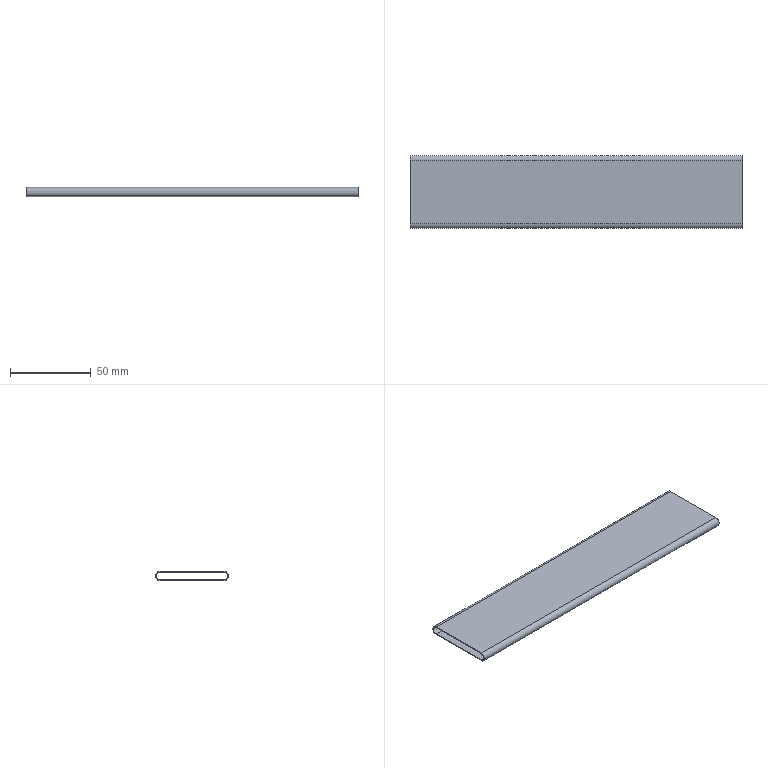Part | STEP file | Tube feed_id914_x_t | 1 solid | 10 faces | box 205 x 45.1 x 5.7 mm | volume 9751 mm3 | plane 6 | cylinder 4 | commonest cylinder face diameters 4.7 x2 5.7 x2
STEP:
#1=CARTESIAN_POINT('',(0.,0.,0.));
#2=DIRECTION('',(0.,0.,1.));
#3=DIRECTION('',(1.,0.,0.));
#4=AXIS2_PLACEMENT_3D('',#1,#2,#3);
#5=CARTESIAN_POINT('',(-74.,-9.664,-6.));
#6=VERTEX_POINT('',#5);
#7=CARTESIAN_POINT('',(-74.,29.736,-6.));
#8=VERTEX_POINT('',#7);
#9=CARTESIAN_POINT('',(-74.,-9.664,-6.));
#10=DIRECTION('',(0.,1.,0.));
#11=VECTOR('',#10,1.);
#12=LINE('',#9,#11);
#13=CARTESIAN_POINT('',(231.,-9.664,-6.));
#14=DIRECTION('',(0.,0.,1.));
#15=DIRECTION('',(0.,-1.,0.));
#16=AXIS2_PLACEMENT_3D('',#13,#14,#15);
#17=PLANE('',#16);
#18=CARTESIAN_POINT('',(0.,-305.));
#19=DIRECTION('',(-1.,0.));
#20=VECTOR('',#19,1.);
#21=LINE('',#18,#20);
#22=(GEOMETRIC_REPRESENTATION_CONTEXT(2)PARAMETRIC_REPRESENTATION_CONTEXT()REPRESENTATION_CONTEXT('',''));
#23=DEFINITIONAL_REPRESENTATION('',(#21),#22);
#24=PCURVE('',#17,#23);
#25=CARTESIAN_POINT('',(-74.,29.736,-3.15));
#26=DIRECTION('',(1.,0.,0.));
#27=DIRECTION('',(0.,0.,-1.));
#28=AXIS2_PLACEMENT_3D('',#25,#26,#27);
#29=PLANE('',#28);
#30=CARTESIAN_POINT('',(2.85,-39.4));
#31=DIRECTION('',(0.,1.));
#32=VECTOR('',#31,1.);
#33=LINE('',#30,#32);
#34=(GEOMETRIC_REPRESENTATION_CONTEXT(2)PARAMETRIC_REPRESENTATION_CONTEXT()REPRESENTATION_CONTEXT('',''));
#35=DEFINITIONAL_REPRESENTATION('',(#33),#34);
#36=PCURVE('',#29,#35);
#37=SURFACE_CURVE('',#12,(#24,#36),.PCURVE_S1.);
#38=EDGE_CURVE('',#6,#8,#37,.T.);
#39=ORIENTED_EDGE('',*,*,#38,.T.);
#40=CARTESIAN_POINT('',(131.,29.736,-6.));
#41=VERTEX_POINT('',#40);
#42=CARTESIAN_POINT('',(231.,29.736,-6.));
#43=DIRECTION('',(-1.,0.,0.));
#44=VECTOR('',#43,1.);
#45=LINE('',#42,#44);
#46=CARTESIAN_POINT('',(-39.4,0.));
#47=DIRECTION('',(0.,-1.));
#48=VECTOR('',#47,1.);
#49=LINE('',#46,#48);
#50=(GEOMETRIC_REPRESENTATION_CONTEXT(2)PARAMETRIC_REPRESENTATION_CONTEXT()REPRESENTATION_CONTEXT('',''));
#51=DEFINITIONAL_REPRESENTATION('',(#49),#50);
#52=PCURVE('',#17,#51);
#53=CARTESIAN_POINT('',(231.,29.736,-3.15));
#54=DIRECTION('',(-1.,0.,0.));
#55=DIRECTION('',(0.,-1.,0.));
#56=AXIS2_PLACEMENT_3D('',#53,#54,#55);
#57=CYLINDRICAL_SURFACE('',#56,2.85);
#58=CARTESIAN_POINT('',(4.712,0.));
#59=DIRECTION('',(0.,1.));
#60=VECTOR('',#59,1.);
#61=LINE('',#58,#60);
#62=(GEOMETRIC_REPRESENTATION_CONTEXT(2)PARAMETRIC_REPRESENTATION_CONTEXT()REPRESENTATION_CONTEXT('',''));
#63=DEFINITIONAL_REPRESENTATION('',(#61),#62);
#64=PCURVE('',#57,#63);
#65=SURFACE_CURVE('',#45,(#52,#64),.PCURVE_S1.);
#66=EDGE_CURVE('',#41,#8,#65,.T.);
#67=ORIENTED_EDGE('',*,*,#66,.F.);
#68=CARTESIAN_POINT('',(131.,-9.664,-6.));
#69=VERTEX_POINT('',#68);
#70=CARTESIAN_POINT('',(131.,-9.664,-6.));
#71=DIRECTION('',(0.,1.,0.));
#72=VECTOR('',#71,1.);
#73=LINE('',#70,#72);
#74=CARTESIAN_POINT('',(0.,-100.));
#75=DIRECTION('',(-1.,0.));
#76=VECTOR('',#75,1.);
#77=LINE('',#74,#76);
#78=(GEOMETRIC_REPRESENTATION_CONTEXT(2)PARAMETRIC_REPRESENTATION_CONTEXT()REPRESENTATION_CONTEXT('',''));
#79=DEFINITIONAL_REPRESENTATION('',(#77),#78);
#80=PCURVE('',#17,#79);
#81=CARTESIAN_POINT('',(131.,29.736,-3.15));
#82=DIRECTION('',(1.,0.,0.));
#83=DIRECTION('',(0.,0.,-1.));
#84=AXIS2_PLACEMENT_3D('',#81,#82,#83);
#85=PLANE('',#84);
#86=CARTESIAN_POINT('',(2.85,-39.4));
#87=DIRECTION('',(0.,1.));
#88=VECTOR('',#87,1.);
#89=LINE('',#86,#88);
#90=(GEOMETRIC_REPRESENTATION_CONTEXT(2)PARAMETRIC_REPRESENTATION_CONTEXT()REPRESENTATION_CONTEXT('',''));
#91=DEFINITIONAL_REPRESENTATION('',(#89),#90);
#92=PCURVE('',#85,#91);
#93=SURFACE_CURVE('',#73,(#80,#92),.PCURVE_S1.);
#94=EDGE_CURVE('',#69,#41,#93,.T.);
#95=ORIENTED_EDGE('',*,*,#94,.F.);
#96=CARTESIAN_POINT('',(231.,-9.664,-6.));
#97=DIRECTION('',(-1.,0.,0.));
#98=VECTOR('',#97,1.);
#99=LINE('',#96,#98);
#100=CARTESIAN_POINT('',(0.,0.));
#101=DIRECTION('',(0.,-1.));
#102=VECTOR('',#101,1.);
#103=LINE('',#100,#102);
#104=(GEOMETRIC_REPRESENTATION_CONTEXT(2)PARAMETRIC_REPRESENTATION_CONTEXT()REPRESENTATION_CONTEXT('',''));
#105=DEFINITIONAL_REPRESENTATION('',(#103),#104);
#106=PCURVE('',#17,#105);
#107=CARTESIAN_POINT('',(231.,-9.664,-3.15));
#108=DIRECTION('',(-1.,0.,0.));
#109=DIRECTION('',(0.,-1.,0.));
#110=AXIS2_PLACEMENT_3D('',#107,#108,#109);
#111=CYLINDRICAL_SURFACE('',#110,2.85);
#112=CARTESIAN_POINT('',(-1.571,0.));
#113=DIRECTION('',(0.,1.));
#114=VECTOR('',#113,1.);
#115=LINE('',#112,#114);
#116=(GEOMETRIC_REPRESENTATION_CONTEXT(2)PARAMETRIC_REPRESENTATION_CONTEXT()REPRESENTATION_CONTEXT('',''));
#117=DEFINITIONAL_REPRESENTATION('',(#115),#116);
#118=PCURVE('',#111,#117);
#119=SURFACE_CURVE('',#99,(#106,#118),.PCURVE_S1.);
#120=EDGE_CURVE('',#69,#6,#119,.T.);
#121=ORIENTED_EDGE('',*,*,#120,.T.);
#122=EDGE_LOOP('',(#39,#67,#95,#121));
#123=FACE_BOUND('',#122,.T.);
#124=ADVANCED_FACE('',(#123),#17,.F.);
#125=CARTESIAN_POINT('',(-74.,29.736,-0.3));
#126=VERTEX_POINT('',#125);
#127=CARTESIAN_POINT('',(-74.,29.736,-3.15));
#128=DIRECTION('',(1.,0.,0.));
#129=DIRECTION('',(0.,1.,0.));
#130=AXIS2_PLACEMENT_3D('',#127,#128,#129);
#131=CIRCLE('',#130,2.85);
#132=CARTESIAN_POINT('',(9.425,305.));
#133=DIRECTION('',(-1.,0.));
#134=VECTOR('',#133,1.);
#135=LINE('',#132,#134);
#136=(GEOMETRIC_REPRESENTATION_CONTEXT(2)PARAMETRIC_REPRESENTATION_CONTEXT()REPRESENTATION_CONTEXT('',''));
#137=DEFINITIONAL_REPRESENTATION('',(#135),#136);
#138=PCURVE('',#57,#137);
#139=CARTESIAN_POINT('',(0.,0.));
#140=DIRECTION('',(0.,1.));
#141=AXIS2_PLACEMENT_2D('',#139,#140);
#142=CIRCLE('',#141,2.85);
#143=(GEOMETRIC_REPRESENTATION_CONTEXT(2)PARAMETRIC_REPRESENTATION_CONTEXT()REPRESENTATION_CONTEXT('',''));
#144=DEFINITIONAL_REPRESENTATION('',(#142),#143);
#145=PCURVE('',#29,#144);
#146=SURFACE_CURVE('',#131,(#138,#145),.PCURVE_S1.);
#147=EDGE_CURVE('',#8,#126,#146,.T.);
#148=ORIENTED_EDGE('',*,*,#147,.T.);
#149=CARTESIAN_POINT('',(131.,29.736,-0.3));
#150=VERTEX_POINT('',#149);
#151=CARTESIAN_POINT('',(231.,29.736,-0.3));
#152=DIRECTION('',(-1.,0.,0.));
#153=VECTOR('',#152,1.);
#154=LINE('',#151,#153);
#155=CARTESIAN_POINT('',(1.571,0.));
#156=DIRECTION('',(0.,1.));
#157=VECTOR('',#156,1.);
#158=LINE('',#155,#157);
#159=(GEOMETRIC_REPRESENTATION_CONTEXT(2)PARAMETRIC_REPRESENTATION_CONTEXT()REPRESENTATION_CONTEXT('',''));
#160=DEFINITIONAL_REPRESENTATION('',(#158),#159);
#161=PCURVE('',#57,#160);
#162=CARTESIAN_POINT('',(231.,29.736,-0.3));
#163=DIRECTION('',(0.,0.,-1.));
#164=DIRECTION('',(0.,1.,0.));
#165=AXIS2_PLACEMENT_3D('',#162,#163,#164);
#166=PLANE('',#165);
#167=CARTESIAN_POINT('',(0.,0.));
#168=DIRECTION('',(0.,-1.));
#169=VECTOR('',#168,1.);
#170=LINE('',#167,#169);
#171=(GEOMETRIC_REPRESENTATION_CONTEXT(2)PARAMETRIC_REPRESENTATION_CONTEXT()REPRESENTATION_CONTEXT('',''));
#172=DEFINITIONAL_REPRESENTATION('',(#170),#171);
#173=PCURVE('',#166,#172);
#174=SURFACE_CURVE('',#154,(#161,#173),.PCURVE_S1.);
#175=EDGE_CURVE('',#150,#126,#174,.T.);
#176=ORIENTED_EDGE('',*,*,#175,.F.);
#177=CARTESIAN_POINT('',(131.,29.736,-3.15));
#178=DIRECTION('',(1.,0.,0.));
#179=DIRECTION('',(0.,0.,-1.));
#180=AXIS2_PLACEMENT_3D('',#177,#178,#179);
#181=CIRCLE('',#180,2.85);
#182=CARTESIAN_POINT('',(4.712,100.));
#183=DIRECTION('',(-1.,0.));
#184=VECTOR('',#183,1.);
#185=LINE('',#182,#184);
#186=(GEOMETRIC_REPRESENTATION_CONTEXT(2)PARAMETRIC_REPRESENTATION_CONTEXT()REPRESENTATION_CONTEXT('',''));
#187=DEFINITIONAL_REPRESENTATION('',(#185),#186);
#188=PCURVE('',#57,#187);
#189=CARTESIAN_POINT('',(0.,0.));
#190=DIRECTION('',(1.,0.));
#191=AXIS2_PLACEMENT_2D('',#189,#190);
#192=CIRCLE('',#191,2.85);
#193=(GEOMETRIC_REPRESENTATION_CONTEXT(2)PARAMETRIC_REPRESENTATION_CONTEXT()REPRESENTATION_CONTEXT('',''));
#194=DEFINITIONAL_REPRESENTATION('',(#192),#193);
#195=PCURVE('',#85,#194);
#196=SURFACE_CURVE('',#181,(#188,#195),.PCURVE_S1.);
#197=EDGE_CURVE('',#41,#150,#196,.T.);
#198=ORIENTED_EDGE('',*,*,#197,.F.);
#199=ORIENTED_EDGE('',*,*,#66,.T.);
#200=EDGE_LOOP('',(#148,#176,#198,#199));
#201=FACE_BOUND('',#200,.T.);
#202=ADVANCED_FACE('',(#201),#57,.T.);
#203=CARTESIAN_POINT('',(-74.,-9.664,-0.3));
#204=VERTEX_POINT('',#203);
#205=CARTESIAN_POINT('',(-74.,29.736,-0.3));
#206=DIRECTION('',(0.,-1.,0.));
#207=VECTOR('',#206,1.);
#208=LINE('',#205,#207);
#209=CARTESIAN_POINT('',(0.,-305.));
#210=DIRECTION('',(-1.,0.));
#211=VECTOR('',#210,1.);
#212=LINE('',#209,#211);
#213=(GEOMETRIC_REPRESENTATION_CONTEXT(2)PARAMETRIC_REPRESENTATION_CONTEXT()REPRESENTATION_CONTEXT('',''));
#214=DEFINITIONAL_REPRESENTATION('',(#212),#213);
#215=PCURVE('',#166,#214);
#216=CARTESIAN_POINT('',(-2.85,0.));
#217=DIRECTION('',(0.,-1.));
#218=VECTOR('',#217,1.);
#219=LINE('',#216,#218);
#220=(GEOMETRIC_REPRESENTATION_CONTEXT(2)PARAMETRIC_REPRESENTATION_CONTEXT()REPRESENTATION_CONTEXT('',''));
#221=DEFINITIONAL_REPRESENTATION('',(#219),#220);
#222=PCURVE('',#29,#221);
#223=SURFACE_CURVE('',#208,(#215,#222),.PCURVE_S1.);
#224=EDGE_CURVE('',#126,#204,#223,.T.);
#225=ORIENTED_EDGE('',*,*,#224,.T.);
#226=CARTESIAN_POINT('',(131.,-9.664,-0.3));
#227=VERTEX_POINT('',#226);
#228=CARTESIAN_POINT('',(231.,-9.664,-0.3));
#229=DIRECTION('',(-1.,0.,0.));
#230=VECTOR('',#229,1.);
#231=LINE('',#228,#230);
#232=CARTESIAN_POINT('',(-39.4,0.));
#233=DIRECTION('',(0.,-1.));
#234=VECTOR('',#233,1.);
#235=LINE('',#232,#234);
#236=(GEOMETRIC_REPRESENTATION_CONTEXT(2)PARAMETRIC_REPRESENTATION_CONTEXT()REPRESENTATION_CONTEXT('',''));
#237=DEFINITIONAL_REPRESENTATION('',(#235),#236);
#238=PCURVE('',#166,#237);
#239=CARTESIAN_POINT('',(1.571,0.));
#240=DIRECTION('',(0.,1.));
#241=VECTOR('',#240,1.);
#242=LINE('',#239,#241);
#243=(GEOMETRIC_REPRESENTATION_CONTEXT(2)PARAMETRIC_REPRESENTATION_CONTEXT()REPRESENTATION_CONTEXT('',''));
#244=DEFINITIONAL_REPRESENTATION('',(#242),#243);
#245=PCURVE('',#111,#244);
#246=SURFACE_CURVE('',#231,(#238,#245),.PCURVE_S1.);
#247=EDGE_CURVE('',#227,#204,#246,.T.);
#248=ORIENTED_EDGE('',*,*,#247,.F.);
#249=CARTESIAN_POINT('',(131.,29.736,-0.3));
#250=DIRECTION('',(0.,-1.,0.));
#251=VECTOR('',#250,1.);
#252=LINE('',#249,#251);
#253=CARTESIAN_POINT('',(0.,-100.));
#254=DIRECTION('',(-1.,0.));
#255=VECTOR('',#254,1.);
#256=LINE('',#253,#255);
#257=(GEOMETRIC_REPRESENTATION_CONTEXT(2)PARAMETRIC_REPRESENTATION_CONTEXT()REPRESENTATION_CONTEXT('',''));
#258=DEFINITIONAL_REPRESENTATION('',(#256),#257);
#259=PCURVE('',#166,#258);
#260=CARTESIAN_POINT('',(-2.85,0.));
#261=DIRECTION('',(0.,-1.));
#262=VECTOR('',#261,1.);
#263=LINE('',#260,#262);
#264=(GEOMETRIC_REPRESENTATION_CONTEXT(2)PARAMETRIC_REPRESENTATION_CONTEXT()REPRESENTATION_CONTEXT('',''));
#265=DEFINITIONAL_REPRESENTATION('',(#263),#264);
#266=PCURVE('',#85,#265);
#267=SURFACE_CURVE('',#252,(#259,#266),.PCURVE_S1.);
#268=EDGE_CURVE('',#150,#227,#267,.T.);
#269=ORIENTED_EDGE('',*,*,#268,.F.);
#270=ORIENTED_EDGE('',*,*,#175,.T.);
#271=EDGE_LOOP('',(#225,#248,#269,#270));
#272=FACE_BOUND('',#271,.T.);
#273=ADVANCED_FACE('',(#272),#166,.F.);
#274=CARTESIAN_POINT('',(-74.,-9.664,-3.15));
#275=DIRECTION('',(1.,0.,0.));
#276=DIRECTION('',(0.,1.,0.));
#277=AXIS2_PLACEMENT_3D('',#274,#275,#276);
#278=CIRCLE('',#277,2.85);
#279=CARTESIAN_POINT('',(3.142,305.));
#280=DIRECTION('',(-1.,0.));
#281=VECTOR('',#280,1.);
#282=LINE('',#279,#281);
#283=(GEOMETRIC_REPRESENTATION_CONTEXT(2)PARAMETRIC_REPRESENTATION_CONTEXT()REPRESENTATION_CONTEXT('',''));
#284=DEFINITIONAL_REPRESENTATION('',(#282),#283);
#285=PCURVE('',#111,#284);
#286=CARTESIAN_POINT('',(0.,-39.4));
#287=DIRECTION('',(0.,1.));
#288=AXIS2_PLACEMENT_2D('',#286,#287);
#289=CIRCLE('',#288,2.85);
#290=(GEOMETRIC_REPRESENTATION_CONTEXT(2)PARAMETRIC_REPRESENTATION_CONTEXT()REPRESENTATION_CONTEXT('',''));
#291=DEFINITIONAL_REPRESENTATION('',(#289),#290);
#292=PCURVE('',#29,#291);
#293=SURFACE_CURVE('',#278,(#285,#292),.PCURVE_S1.);
#294=EDGE_CURVE('',#204,#6,#293,.T.);
#295=ORIENTED_EDGE('',*,*,#294,.T.);
#296=ORIENTED_EDGE('',*,*,#120,.F.);
#297=CARTESIAN_POINT('',(131.,-9.664,-3.15));
#298=DIRECTION('',(1.,0.,0.));
#299=DIRECTION('',(0.,0.,-1.));
#300=AXIS2_PLACEMENT_3D('',#297,#298,#299);
#301=CIRCLE('',#300,2.85);
#302=CARTESIAN_POINT('',(4.712,100.));
#303=DIRECTION('',(-1.,0.));
#304=VECTOR('',#303,1.);
#305=LINE('',#302,#304);
#306=(GEOMETRIC_REPRESENTATION_CONTEXT(2)PARAMETRIC_REPRESENTATION_CONTEXT()REPRESENTATION_CONTEXT('',''));
#307=DEFINITIONAL_REPRESENTATION('',(#305),#306);
#308=PCURVE('',#111,#307);
#309=CARTESIAN_POINT('',(0.,-39.4));
#310=DIRECTION('',(1.,0.));
#311=AXIS2_PLACEMENT_2D('',#309,#310);
#312=CIRCLE('',#311,2.85);
#313=(GEOMETRIC_REPRESENTATION_CONTEXT(2)PARAMETRIC_REPRESENTATION_CONTEXT()REPRESENTATION_CONTEXT('',''));
#314=DEFINITIONAL_REPRESENTATION('',(#312),#313);
#315=PCURVE('',#85,#314);
#316=SURFACE_CURVE('',#301,(#308,#315),.PCURVE_S1.);
#317=EDGE_CURVE('',#227,#69,#316,.T.);
#318=ORIENTED_EDGE('',*,*,#317,.F.);
#319=ORIENTED_EDGE('',*,*,#247,.T.);
#320=EDGE_LOOP('',(#295,#296,#318,#319));
#321=FACE_BOUND('',#320,.T.);
#322=ADVANCED_FACE('',(#321),#111,.T.);
#323=CARTESIAN_POINT('',(131.,-9.664,-5.5));
#324=VERTEX_POINT('',#323);
#325=CARTESIAN_POINT('',(131.,29.736,-5.5));
#326=VERTEX_POINT('',#325);
#327=CARTESIAN_POINT('',(131.,-9.664,-5.5));
#328=DIRECTION('',(0.,1.,0.));
#329=VECTOR('',#328,1.);
#330=LINE('',#327,#329);
#331=CARTESIAN_POINT('',(2.35,-39.4));
#332=DIRECTION('',(0.,1.));
#333=VECTOR('',#332,1.);
#334=LINE('',#331,#333);
#335=(GEOMETRIC_REPRESENTATION_CONTEXT(2)PARAMETRIC_REPRESENTATION_CONTEXT()REPRESENTATION_CONTEXT('',''));
#336=DEFINITIONAL_REPRESENTATION('',(#334),#335);
#337=PCURVE('',#85,#336);
#338=CARTESIAN_POINT('',(231.,-9.664,-5.5));
#339=DIRECTION('',(0.,0.,1.));
#340=DIRECTION('',(0.,-1.,0.));
#341=AXIS2_PLACEMENT_3D('',#338,#339,#340);
#342=PLANE('',#341);
#343=CARTESIAN_POINT('',(0.,-100.));
#344=DIRECTION('',(-1.,0.));
#345=VECTOR('',#344,1.);
#346=LINE('',#343,#345);
#347=(GEOMETRIC_REPRESENTATION_CONTEXT(2)PARAMETRIC_REPRESENTATION_CONTEXT()REPRESENTATION_CONTEXT('',''));
#348=DEFINITIONAL_REPRESENTATION('',(#346),#347);
#349=PCURVE('',#342,#348);
#350=SURFACE_CURVE('',#330,(#337,#349),.PCURVE_S1.);
#351=EDGE_CURVE('',#324,#326,#350,.T.);
#352=ORIENTED_EDGE('',*,*,#351,.F.);
#353=CARTESIAN_POINT('',(131.,-9.664,-0.8));
#354=VERTEX_POINT('',#353);
#355=CARTESIAN_POINT('',(131.,-9.664,-3.15));
#356=DIRECTION('',(1.,0.,0.));
#357=DIRECTION('',(0.,0.,-1.));
#358=AXIS2_PLACEMENT_3D('',#355,#356,#357);
#359=CIRCLE('',#358,2.35);
#360=CARTESIAN_POINT('',(0.,-39.4));
#361=DIRECTION('',(1.,0.));
#362=AXIS2_PLACEMENT_2D('',#360,#361);
#363=CIRCLE('',#362,2.35);
#364=(GEOMETRIC_REPRESENTATION_CONTEXT(2)PARAMETRIC_REPRESENTATION_CONTEXT()REPRESENTATION_CONTEXT('',''));
#365=DEFINITIONAL_REPRESENTATION('',(#363),#364);
#366=PCURVE('',#85,#365);
#367=CARTESIAN_POINT('',(231.,-9.664,-3.15));
#368=DIRECTION('',(-1.,0.,0.));
#369=DIRECTION('',(0.,-1.,0.));
#370=AXIS2_PLACEMENT_3D('',#367,#368,#369);
#371=CYLINDRICAL_SURFACE('',#370,2.35);
#372=CARTESIAN_POINT('',(10.996,100.));
#373=DIRECTION('',(-1.,0.));
#374=VECTOR('',#373,1.);
#375=LINE('',#372,#374);
#376=(GEOMETRIC_REPRESENTATION_CONTEXT(2)PARAMETRIC_REPRESENTATION_CONTEXT()REPRESENTATION_CONTEXT('',''));
#377=DEFINITIONAL_REPRESENTATION('',(#375),#376);
#378=PCURVE('',#371,#377);
#379=SURFACE_CURVE('',#359,(#366,#378),.PCURVE_S1.);
#380=EDGE_CURVE('',#354,#324,#379,.T.);
#381=ORIENTED_EDGE('',*,*,#380,.F.);
#382=CARTESIAN_POINT('',(131.,29.736,-0.8));
#383=VERTEX_POINT('',#382);
#384=CARTESIAN_POINT('',(131.,29.736,-0.8));
#385=DIRECTION('',(0.,-1.,0.));
#386=VECTOR('',#385,1.);
#387=LINE('',#384,#386);
#388=CARTESIAN_POINT('',(-2.35,0.));
#389=DIRECTION('',(0.,-1.));
#390=VECTOR('',#389,1.);
#391=LINE('',#388,#390);
#392=(GEOMETRIC_REPRESENTATION_CONTEXT(2)PARAMETRIC_REPRESENTATION_CONTEXT()REPRESENTATION_CONTEXT('',''));
#393=DEFINITIONAL_REPRESENTATION('',(#391),#392);
#394=PCURVE('',#85,#393);
#395=CARTESIAN_POINT('',(231.,29.736,-0.8));
#396=DIRECTION('',(0.,0.,-1.));
#397=DIRECTION('',(0.,1.,0.));
#398=AXIS2_PLACEMENT_3D('',#395,#396,#397);
#399=PLANE('',#398);
#400=CARTESIAN_POINT('',(0.,-100.));
#401=DIRECTION('',(-1.,0.));
#402=VECTOR('',#401,1.);
#403=LINE('',#400,#402);
#404=(GEOMETRIC_REPRESENTATION_CONTEXT(2)PARAMETRIC_REPRESENTATION_CONTEXT()REPRESENTATION_CONTEXT('',''));
#405=DEFINITIONAL_REPRESENTATION('',(#403),#404);
#406=PCURVE('',#399,#405);
#407=SURFACE_CURVE('',#387,(#394,#406),.PCURVE_S1.);
#408=EDGE_CURVE('',#383,#354,#407,.T.);
#409=ORIENTED_EDGE('',*,*,#408,.F.);
#410=CARTESIAN_POINT('',(131.,29.736,-3.15));
#411=DIRECTION('',(1.,0.,0.));
#412=DIRECTION('',(0.,0.,-1.));
#413=AXIS2_PLACEMENT_3D('',#410,#411,#412);
#414=CIRCLE('',#413,2.35);
#415=CARTESIAN_POINT('',(0.,0.));
#416=DIRECTION('',(1.,0.));
#417=AXIS2_PLACEMENT_2D('',#415,#416);
#418=CIRCLE('',#417,2.35);
#419=(GEOMETRIC_REPRESENTATION_CONTEXT(2)PARAMETRIC_REPRESENTATION_CONTEXT()REPRESENTATION_CONTEXT('',''));
#420=DEFINITIONAL_REPRESENTATION('',(#418),#419);
#421=PCURVE('',#85,#420);
#422=CARTESIAN_POINT('',(231.,29.736,-3.15));
#423=DIRECTION('',(-1.,0.,0.));
#424=DIRECTION('',(0.,-1.,0.));
#425=AXIS2_PLACEMENT_3D('',#422,#423,#424);
#426=CYLINDRICAL_SURFACE('',#425,2.35);
#427=CARTESIAN_POINT('',(4.712,100.));
#428=DIRECTION('',(-1.,0.));
#429=VECTOR('',#428,1.);
#430=LINE('',#427,#429);
#431=(GEOMETRIC_REPRESENTATION_CONTEXT(2)PARAMETRIC_REPRESENTATION_CONTEXT()REPRESENTATION_CONTEXT('',''));
#432=DEFINITIONAL_REPRESENTATION('',(#430),#431);
#433=PCURVE('',#426,#432);
#434=SURFACE_CURVE('',#414,(#421,#433),.PCURVE_S1.);
#435=EDGE_CURVE('',#326,#383,#434,.T.);
#436=ORIENTED_EDGE('',*,*,#435,.F.);
#437=EDGE_LOOP('',(#352,#381,#409,#436));
#438=FACE_BOUND('',#437,.T.);
#439=ORIENTED_EDGE('',*,*,#94,.T.);
#440=ORIENTED_EDGE('',*,*,#197,.T.);
#441=ORIENTED_EDGE('',*,*,#268,.T.);
#442=ORIENTED_EDGE('',*,*,#317,.T.);
#443=EDGE_LOOP('',(#439,#440,#441,#442));
#444=FACE_BOUND('',#443,.T.);
#445=ADVANCED_FACE('',(#438,#444),#85,.T.);
#446=CARTESIAN_POINT('',(-74.,-9.664,-0.8));
#447=VERTEX_POINT('',#446);
#448=CARTESIAN_POINT('',(-74.,-9.664,-5.5));
#449=VERTEX_POINT('',#448);
#450=CARTESIAN_POINT('',(-74.,-9.664,-3.15));
#451=DIRECTION('',(1.,0.,0.));
#452=DIRECTION('',(0.,0.,-1.));
#453=AXIS2_PLACEMENT_3D('',#450,#451,#452);
#454=CIRCLE('',#453,2.35);
#455=CARTESIAN_POINT('',(0.,-39.4));
#456=DIRECTION('',(1.,0.));
#457=AXIS2_PLACEMENT_2D('',#455,#456);
#458=CIRCLE('',#457,2.35);
#459=(GEOMETRIC_REPRESENTATION_CONTEXT(2)PARAMETRIC_REPRESENTATION_CONTEXT()REPRESENTATION_CONTEXT('',''));
#460=DEFINITIONAL_REPRESENTATION('',(#458),#459);
#461=PCURVE('',#29,#460);
#462=CARTESIAN_POINT('',(10.996,305.));
#463=DIRECTION('',(-1.,0.));
#464=VECTOR('',#463,1.);
#465=LINE('',#462,#464);
#466=(GEOMETRIC_REPRESENTATION_CONTEXT(2)PARAMETRIC_REPRESENTATION_CONTEXT()REPRESENTATION_CONTEXT('',''));
#467=DEFINITIONAL_REPRESENTATION('',(#465),#466);
#468=PCURVE('',#371,#467);
#469=SURFACE_CURVE('',#454,(#461,#468),.PCURVE_S1.);
#470=EDGE_CURVE('',#447,#449,#469,.T.);
#471=ORIENTED_EDGE('',*,*,#470,.T.);
#472=CARTESIAN_POINT('',(-74.,29.736,-5.5));
#473=VERTEX_POINT('',#472);
#474=CARTESIAN_POINT('',(-74.,-9.664,-5.5));
#475=DIRECTION('',(0.,1.,0.));
#476=VECTOR('',#475,1.);
#477=LINE('',#474,#476);
#478=CARTESIAN_POINT('',(2.35,-39.4));
#479=DIRECTION('',(0.,1.));
#480=VECTOR('',#479,1.);
#481=LINE('',#478,#480);
#482=(GEOMETRIC_REPRESENTATION_CONTEXT(2)PARAMETRIC_REPRESENTATION_CONTEXT()REPRESENTATION_CONTEXT('',''));
#483=DEFINITIONAL_REPRESENTATION('',(#481),#482);
#484=PCURVE('',#29,#483);
#485=CARTESIAN_POINT('',(0.,-305.));
#486=DIRECTION('',(-1.,0.));
#487=VECTOR('',#486,1.);
#488=LINE('',#485,#487);
#489=(GEOMETRIC_REPRESENTATION_CONTEXT(2)PARAMETRIC_REPRESENTATION_CONTEXT()REPRESENTATION_CONTEXT('',''));
#490=DEFINITIONAL_REPRESENTATION('',(#488),#489);
#491=PCURVE('',#342,#490);
#492=SURFACE_CURVE('',#477,(#484,#491),.PCURVE_S1.);
#493=EDGE_CURVE('',#449,#473,#492,.T.);
#494=ORIENTED_EDGE('',*,*,#493,.T.);
#495=CARTESIAN_POINT('',(-74.,29.736,-0.8));
#496=VERTEX_POINT('',#495);
#497=CARTESIAN_POINT('',(-74.,29.736,-3.15));
#498=DIRECTION('',(1.,0.,0.));
#499=DIRECTION('',(0.,0.,-1.));
#500=AXIS2_PLACEMENT_3D('',#497,#498,#499);
#501=CIRCLE('',#500,2.35);
#502=CARTESIAN_POINT('',(0.,0.));
#503=DIRECTION('',(1.,0.));
#504=AXIS2_PLACEMENT_2D('',#502,#503);
#505=CIRCLE('',#504,2.35);
#506=(GEOMETRIC_REPRESENTATION_CONTEXT(2)PARAMETRIC_REPRESENTATION_CONTEXT()REPRESENTATION_CONTEXT('',''));
#507=DEFINITIONAL_REPRESENTATION('',(#505),#506);
#508=PCURVE('',#29,#507);
#509=CARTESIAN_POINT('',(4.712,305.));
#510=DIRECTION('',(-1.,0.));
#511=VECTOR('',#510,1.);
#512=LINE('',#509,#511);
#513=(GEOMETRIC_REPRESENTATION_CONTEXT(2)PARAMETRIC_REPRESENTATION_CONTEXT()REPRESENTATION_CONTEXT('',''));
#514=DEFINITIONAL_REPRESENTATION('',(#512),#513);
#515=PCURVE('',#426,#514);
#516=SURFACE_CURVE('',#501,(#508,#515),.PCURVE_S1.);
#517=EDGE_CURVE('',#473,#496,#516,.T.);
#518=ORIENTED_EDGE('',*,*,#517,.T.);
#519=CARTESIAN_POINT('',(-74.,29.736,-0.8));
#520=DIRECTION('',(0.,-1.,0.));
#521=VECTOR('',#520,1.);
#522=LINE('',#519,#521);
#523=CARTESIAN_POINT('',(-2.35,0.));
#524=DIRECTION('',(0.,-1.));
#525=VECTOR('',#524,1.);
#526=LINE('',#523,#525);
#527=(GEOMETRIC_REPRESENTATION_CONTEXT(2)PARAMETRIC_REPRESENTATION_CONTEXT()REPRESENTATION_CONTEXT('',''));
#528=DEFINITIONAL_REPRESENTATION('',(#526),#527);
#529=PCURVE('',#29,#528);
#530=CARTESIAN_POINT('',(0.,-305.));
#531=DIRECTION('',(-1.,0.));
#532=VECTOR('',#531,1.);
#533=LINE('',#530,#532);
#534=(GEOMETRIC_REPRESENTATION_CONTEXT(2)PARAMETRIC_REPRESENTATION_CONTEXT()REPRESENTATION_CONTEXT('',''));
#535=DEFINITIONAL_REPRESENTATION('',(#533),#534);
#536=PCURVE('',#399,#535);
#537=SURFACE_CURVE('',#522,(#529,#536),.PCURVE_S1.);
#538=EDGE_CURVE('',#496,#447,#537,.T.);
#539=ORIENTED_EDGE('',*,*,#538,.T.);
#540=EDGE_LOOP('',(#471,#494,#518,#539));
#541=FACE_BOUND('',#540,.T.);
#542=ORIENTED_EDGE('',*,*,#38,.F.);
#543=ORIENTED_EDGE('',*,*,#294,.F.);
#544=ORIENTED_EDGE('',*,*,#224,.F.);
#545=ORIENTED_EDGE('',*,*,#147,.F.);
#546=EDGE_LOOP('',(#542,#543,#544,#545));
#547=FACE_BOUND('',#546,.T.);
#548=ADVANCED_FACE('',(#541,#547),#29,.F.);
#549=ORIENTED_EDGE('',*,*,#493,.F.);
#550=CARTESIAN_POINT('',(231.,-9.664,-5.5));
#551=DIRECTION('',(-1.,0.,0.));
#552=VECTOR('',#551,1.);
#553=LINE('',#550,#552);
#554=CARTESIAN_POINT('',(0.,0.));
#555=DIRECTION('',(0.,-1.));
#556=VECTOR('',#555,1.);
#557=LINE('',#554,#556);
#558=(GEOMETRIC_REPRESENTATION_CONTEXT(2)PARAMETRIC_REPRESENTATION_CONTEXT()REPRESENTATION_CONTEXT('',''));
#559=DEFINITIONAL_REPRESENTATION('',(#557),#558);
#560=PCURVE('',#342,#559);
#561=CARTESIAN_POINT('',(4.712,0.));
#562=DIRECTION('',(0.,1.));
#563=VECTOR('',#562,1.);
#564=LINE('',#561,#563);
#565=(GEOMETRIC_REPRESENTATION_CONTEXT(2)PARAMETRIC_REPRESENTATION_CONTEXT()REPRESENTATION_CONTEXT('',''));
#566=DEFINITIONAL_REPRESENTATION('',(#564),#565);
#567=PCURVE('',#371,#566);
#568=SURFACE_CURVE('',#553,(#560,#567),.PCURVE_S1.);
#569=EDGE_CURVE('',#324,#449,#568,.T.);
#570=ORIENTED_EDGE('',*,*,#569,.F.);
#571=ORIENTED_EDGE('',*,*,#351,.T.);
#572=CARTESIAN_POINT('',(231.,29.736,-5.5));
#573=DIRECTION('',(-1.,0.,0.));
#574=VECTOR('',#573,1.);
#575=LINE('',#572,#574);
#576=CARTESIAN_POINT('',(-39.4,0.));
#577=DIRECTION('',(0.,-1.));
#578=VECTOR('',#577,1.);
#579=LINE('',#576,#578);
#580=(GEOMETRIC_REPRESENTATION_CONTEXT(2)PARAMETRIC_REPRESENTATION_CONTEXT()REPRESENTATION_CONTEXT('',''));
#581=DEFINITIONAL_REPRESENTATION('',(#579),#580);
#582=PCURVE('',#342,#581);
#583=CARTESIAN_POINT('',(4.712,0.));
#584=DIRECTION('',(0.,1.));
#585=VECTOR('',#584,1.);
#586=LINE('',#583,#585);
#587=(GEOMETRIC_REPRESENTATION_CONTEXT(2)PARAMETRIC_REPRESENTATION_CONTEXT()REPRESENTATION_CONTEXT('',''));
#588=DEFINITIONAL_REPRESENTATION('',(#586),#587);
#589=PCURVE('',#426,#588);
#590=SURFACE_CURVE('',#575,(#582,#589),.PCURVE_S1.);
#591=EDGE_CURVE('',#326,#473,#590,.T.);
#592=ORIENTED_EDGE('',*,*,#591,.T.);
#593=EDGE_LOOP('',(#549,#570,#571,#592));
#594=FACE_BOUND('',#593,.T.);
#595=ADVANCED_FACE('',(#594),#342,.T.);
#596=CARTESIAN_POINT('',(231.,29.736,-0.8));
#597=DIRECTION('',(-1.,0.,0.));
#598=VECTOR('',#597,1.);
#599=LINE('',#596,#598);
#600=CARTESIAN_POINT('',(1.571,0.));
#601=DIRECTION('',(0.,1.));
#602=VECTOR('',#601,1.);
#603=LINE('',#600,#602);
#604=(GEOMETRIC_REPRESENTATION_CONTEXT(2)PARAMETRIC_REPRESENTATION_CONTEXT()REPRESENTATION_CONTEXT('',''));
#605=DEFINITIONAL_REPRESENTATION('',(#603),#604);
#606=PCURVE('',#426,#605);
#607=CARTESIAN_POINT('',(0.,0.));
#608=DIRECTION('',(0.,-1.));
#609=VECTOR('',#608,1.);
#610=LINE('',#607,#609);
#611=(GEOMETRIC_REPRESENTATION_CONTEXT(2)PARAMETRIC_REPRESENTATION_CONTEXT()REPRESENTATION_CONTEXT('',''));
#612=DEFINITIONAL_REPRESENTATION('',(#610),#611);
#613=PCURVE('',#399,#612);
#614=SURFACE_CURVE('',#599,(#606,#613),.PCURVE_S1.);
#615=EDGE_CURVE('',#383,#496,#614,.T.);
#616=ORIENTED_EDGE('',*,*,#615,.F.);
#617=ORIENTED_EDGE('',*,*,#435,.F.);
#618=ORIENTED_EDGE('',*,*,#591,.T.);
#619=ORIENTED_EDGE('',*,*,#517,.T.);
#620=EDGE_LOOP('',(#616,#617,#618,#619));
#621=FACE_BOUND('',#620,.F.);
#622=ADVANCED_FACE('',(#621),#426,.F.);
#623=ORIENTED_EDGE('',*,*,#538,.F.);
#624=ORIENTED_EDGE('',*,*,#615,.F.);
#625=ORIENTED_EDGE('',*,*,#408,.T.);
#626=CARTESIAN_POINT('',(231.,-9.664,-0.8));
#627=DIRECTION('',(-1.,0.,0.));
#628=VECTOR('',#627,1.);
#629=LINE('',#626,#628);
#630=CARTESIAN_POINT('',(-39.4,0.));
#631=DIRECTION('',(0.,-1.));
#632=VECTOR('',#631,1.);
#633=LINE('',#630,#632);
#634=(GEOMETRIC_REPRESENTATION_CONTEXT(2)PARAMETRIC_REPRESENTATION_CONTEXT()REPRESENTATION_CONTEXT('',''));
#635=DEFINITIONAL_REPRESENTATION('',(#633),#634);
#636=PCURVE('',#399,#635);
#637=CARTESIAN_POINT('',(7.854,0.));
#638=DIRECTION('',(0.,1.));
#639=VECTOR('',#638,1.);
#640=LINE('',#637,#639);
#641=(GEOMETRIC_REPRESENTATION_CONTEXT(2)PARAMETRIC_REPRESENTATION_CONTEXT()REPRESENTATION_CONTEXT('',''));
#642=DEFINITIONAL_REPRESENTATION('',(#640),#641);
#643=PCURVE('',#371,#642);
#644=SURFACE_CURVE('',#629,(#636,#643),.PCURVE_S1.);
#645=EDGE_CURVE('',#354,#447,#644,.T.);
#646=ORIENTED_EDGE('',*,*,#645,.T.);
#647=EDGE_LOOP('',(#623,#624,#625,#646));
#648=FACE_BOUND('',#647,.T.);
#649=ADVANCED_FACE('',(#648),#399,.T.);
#650=ORIENTED_EDGE('',*,*,#569,.F.);
#651=ORIENTED_EDGE('',*,*,#380,.F.);
#652=ORIENTED_EDGE('',*,*,#645,.T.);
#653=ORIENTED_EDGE('',*,*,#470,.T.);
#654=EDGE_LOOP('',(#650,#651,#652,#653));
#655=FACE_BOUND('',#654,.F.);
#656=ADVANCED_FACE('',(#655),#371,.F.);
#657=CLOSED_SHELL('',(#124,#202,#273,#322,#445,#548,#595,#622,#649,#656));
#658=MANIFOLD_SOLID_BREP('',#657);
#659=(LENGTH_UNIT()NAMED_UNIT(*)SI_UNIT(.MILLI.,.METRE.));
#660=UNCERTAINTY_MEASURE_WITH_UNIT(LENGTH_MEASURE(0.0000001),#659,'','');
#661=(NAMED_UNIT(*)PLANE_ANGLE_UNIT()SI_UNIT($,.RADIAN.));
#662=(NAMED_UNIT(*)SI_UNIT($,.STERADIAN.)SOLID_ANGLE_UNIT());
#663=(GEOMETRIC_REPRESENTATION_CONTEXT(3)GLOBAL_UNCERTAINTY_ASSIGNED_CONTEXT((#660))GLOBAL_UNIT_ASSIGNED_CONTEXT((#659,#661,#662))REPRESENTATION_CONTEXT('',''));
#664=ADVANCED_BREP_SHAPE_REPRESENTATION('',(#4,#658),#663);